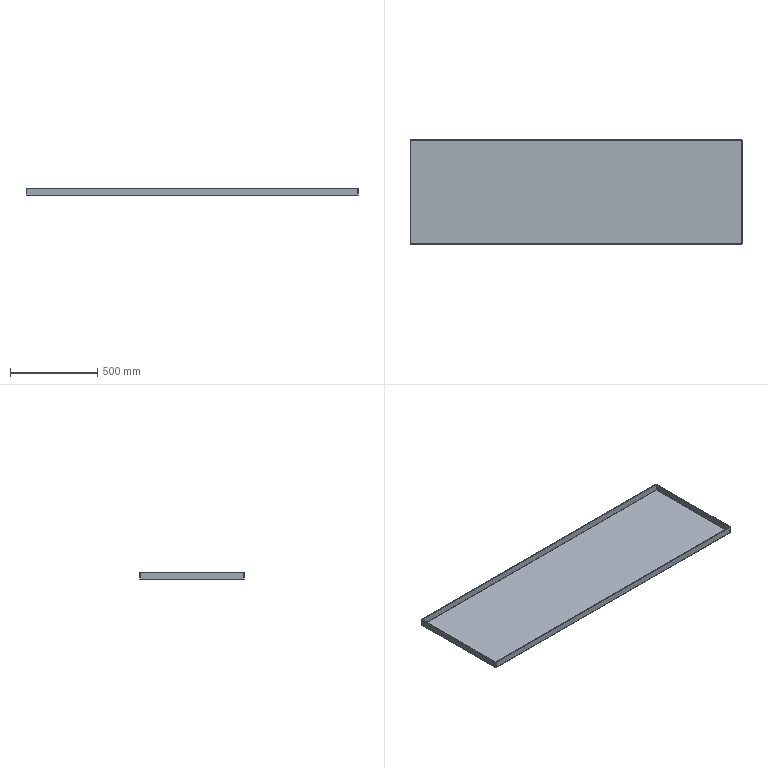Part | SolidWorks | features EdgeFlange 1, FlatPattern 1, SMBaseFlange 1, SheetMetal 1 | 1 solid | 38 faces | box 1900 x 600 x 40 mm | volume 2650874 mm3 | plane 22 | spline 8 | cylinder 8 | commonest cylinder face diameters 1.473 x4 5.473 x4
STEP:
#1=CARTESIAN_POINT('',(947.263,297.263,-2.));
#2=VERTEX_POINT('',#1);
#3=CARTESIAN_POINT('',(947.263,-297.263,-2.));
#4=VERTEX_POINT('',#3);
#5=CARTESIAN_POINT('',(947.263,297.293,-2.));
#6=DIRECTION('',(0.,-1.,0.));
#7=VECTOR('',#6,1000.);
#8=LINE('',#5,#7);
#9=EDGE_CURVE('',#2,#4,#8,.T.);
#10=ORIENTED_EDGE('',*,*,#9,.T.);
#11=CARTESIAN_POINT('',(-947.263,-297.263,-2.));
#12=VERTEX_POINT('',#11);
#13=CARTESIAN_POINT('',(947.293,-297.263,-2.));
#14=DIRECTION('',(-1.,0.,0.));
#15=VECTOR('',#14,1000.);
#16=LINE('',#13,#15);
#17=EDGE_CURVE('',#4,#12,#16,.T.);
#18=ORIENTED_EDGE('',*,*,#17,.T.);
#19=CARTESIAN_POINT('',(-947.263,297.263,-2.));
#20=VERTEX_POINT('',#19);
#21=CARTESIAN_POINT('',(-947.263,-297.293,-2.));
#22=DIRECTION('',(0.,1.,0.));
#23=VECTOR('',#22,1000.);
#24=LINE('',#21,#23);
#25=EDGE_CURVE('',#12,#20,#24,.T.);
#26=ORIENTED_EDGE('',*,*,#25,.T.);
#27=CARTESIAN_POINT('',(-947.293,297.263,-2.));
#28=DIRECTION('',(1.,0.,0.));
#29=VECTOR('',#28,1000.);
#30=LINE('',#27,#29);
#31=EDGE_CURVE('',#20,#2,#30,.T.);
#32=ORIENTED_EDGE('',*,*,#31,.T.);
#33=EDGE_LOOP('',(#10,#18,#26,#32));
#34=FACE_OUTER_BOUND('',#33,.T.);
#35=CARTESIAN_POINT('',(0.,0.,-2.));
#36=DIRECTION('',(0.,0.,-1.));
#37=DIRECTION('',(-1.,0.,0.));
#38=AXIS2_PLACEMENT_3D('',#35,#36,#37);
#39=PLANE('',#38);
#40=ADVANCED_FACE('',(#34),#39,.T.);
#41=CARTESIAN_POINT('',(947.263,-297.263,0.));
#42=VERTEX_POINT('',#41);
#43=CARTESIAN_POINT('',(-947.263,-297.263,0.));
#44=VERTEX_POINT('',#43);
#45=CARTESIAN_POINT('',(947.293,-297.263,0.));
#46=DIRECTION('',(-1.,0.,0.));
#47=VECTOR('',#46,1000.);
#48=LINE('',#45,#47);
#49=EDGE_CURVE('',#42,#44,#48,.T.);
#50=ORIENTED_EDGE('',*,*,#49,.F.);
#51=CARTESIAN_POINT('',(947.263,297.263,0.));
#52=VERTEX_POINT('',#51);
#53=CARTESIAN_POINT('',(947.263,297.293,0.));
#54=DIRECTION('',(0.,-1.,0.));
#55=VECTOR('',#54,1000.);
#56=LINE('',#53,#55);
#57=EDGE_CURVE('',#52,#42,#56,.T.);
#58=ORIENTED_EDGE('',*,*,#57,.F.);
#59=CARTESIAN_POINT('',(-947.263,297.263,0.));
#60=VERTEX_POINT('',#59);
#61=CARTESIAN_POINT('',(-947.293,297.263,0.));
#62=DIRECTION('',(1.,0.,0.));
#63=VECTOR('',#62,1000.);
#64=LINE('',#61,#63);
#65=EDGE_CURVE('',#60,#52,#64,.T.);
#66=ORIENTED_EDGE('',*,*,#65,.F.);
#67=CARTESIAN_POINT('',(-947.263,-297.293,0.));
#68=DIRECTION('',(0.,1.,0.));
#69=VECTOR('',#68,1000.);
#70=LINE('',#67,#69);
#71=EDGE_CURVE('',#44,#60,#70,.T.);
#72=ORIENTED_EDGE('',*,*,#71,.F.);
#73=EDGE_LOOP('',(#50,#58,#66,#72));
#74=FACE_OUTER_BOUND('',#73,.T.);
#75=CARTESIAN_POINT('',(0.,0.,0.));
#76=DIRECTION('',(0.,0.,-1.));
#77=DIRECTION('',(-1.,0.,0.));
#78=AXIS2_PLACEMENT_3D('',#75,#76,#77);
#79=PLANE('',#78);
#80=ADVANCED_FACE('',(#74),#79,.F.);
#81=CARTESIAN_POINT('',(947.293,300.,0.7366));
#82=VERTEX_POINT('',#81);
#83=CARTESIAN_POINT('',(947.293,298.,0.7366));
#84=VERTEX_POINT('',#83);
#85=CARTESIAN_POINT('',(947.293,298.,0.7366));
#86=DIRECTION('',(0.,-1.,0.));
#87=VECTOR('',#86,1000.);
#88=LINE('',#85,#87);
#89=EDGE_CURVE('',#82,#84,#88,.T.);
#90=ORIENTED_EDGE('',*,*,#89,.T.);
#91=CARTESIAN_POINT('',(947.263,297.263,0.));
#92=CARTESIAN_POINT('',(947.268,297.456,0.));
#93=CARTESIAN_POINT('',(947.273,297.648,0.07939));
#94=CARTESIAN_POINT('',(947.283,297.921,0.3521));
#95=CARTESIAN_POINT('',(947.288,298.,0.5438));
#96=CARTESIAN_POINT('',(947.293,298.,0.7366));
#97=B_SPLINE_CURVE_WITH_KNOTS('',3,(#91,#92,#93,#94,#95,#96),.UNSPECIFIED.,.F.,.F.,(4,2,4),(0.,0.5,1.),.UNSPECIFIED.);
#98=EDGE_CURVE('',#52,#84,#97,.T.);
#99=ORIENTED_EDGE('',*,*,#98,.F.);
#100=CARTESIAN_POINT('',(947.263,297.263,0.));
#101=DIRECTION('',(0.,0.,-1.));
#102=VECTOR('',#101,1000.);
#103=LINE('',#100,#102);
#104=EDGE_CURVE('',#52,#2,#103,.T.);
#105=ORIENTED_EDGE('',*,*,#104,.T.);
#106=CARTESIAN_POINT('',(947.263,297.263,-2.));
#107=CARTESIAN_POINT('',(947.266,297.622,-2.));
#108=CARTESIAN_POINT('',(947.268,297.98,-1.929));
#109=CARTESIAN_POINT('',(947.273,298.642,-1.655));
#110=CARTESIAN_POINT('',(947.276,298.945,-1.452));
#111=CARTESIAN_POINT('',(947.281,299.452,-0.9452));
#112=CARTESIAN_POINT('',(947.283,299.655,-0.6416));
#113=CARTESIAN_POINT('',(947.288,299.929,0.0203));
#114=CARTESIAN_POINT('',(947.29,300.,0.3784));
#115=CARTESIAN_POINT('',(947.293,300.,0.7366));
#116=B_SPLINE_CURVE_WITH_KNOTS('',3,(#106,#107,#108,#109,#110,#111,#112,#113,#114,#115),.UNSPECIFIED.,.F.,.F.,(4,2,2,2,4),(0.,0.25,0.5,0.75,1.),.UNSPECIFIED.);
#117=EDGE_CURVE('',#2,#82,#116,.T.);
#118=ORIENTED_EDGE('',*,*,#117,.T.);
#119=EDGE_LOOP('',(#90,#99,#105,#118));
#120=FACE_OUTER_BOUND('',#119,.T.);
#121=CARTESIAN_POINT('',(947.263,297.263,-2.02));
#122=CARTESIAN_POINT('',(947.266,297.624,-2.02));
#123=CARTESIAN_POINT('',(947.268,297.985,-1.948));
#124=CARTESIAN_POINT('',(947.273,298.652,-1.672));
#125=CARTESIAN_POINT('',(947.276,298.957,-1.468));
#126=CARTESIAN_POINT('',(947.281,299.468,-0.9575));
#127=CARTESIAN_POINT('',(947.283,299.672,-0.6517));
#128=CARTESIAN_POINT('',(947.288,299.948,0.01507));
#129=CARTESIAN_POINT('',(947.29,300.02,0.3757));
#130=CARTESIAN_POINT('',(947.293,300.02,0.7366));
#131=CARTESIAN_POINT('',(947.263,297.263,-2.));
#132=CARTESIAN_POINT('',(947.266,297.622,-2.));
#133=CARTESIAN_POINT('',(947.268,297.98,-1.929));
#134=CARTESIAN_POINT('',(947.273,298.642,-1.655));
#135=CARTESIAN_POINT('',(947.276,298.945,-1.452));
#136=CARTESIAN_POINT('',(947.281,299.452,-0.9452));
#137=CARTESIAN_POINT('',(947.283,299.655,-0.6416));
#138=CARTESIAN_POINT('',(947.288,299.929,0.0203));
#139=CARTESIAN_POINT('',(947.29,300.,0.3783));
#140=CARTESIAN_POINT('',(947.293,300.,0.7366));
#141=CARTESIAN_POINT('',(947.263,297.263,0.));
#142=CARTESIAN_POINT('',(947.266,297.36,0.));
#143=CARTESIAN_POINT('',(947.268,297.456,0.01917));
#144=CARTESIAN_POINT('',(947.273,297.634,0.09297));
#145=CARTESIAN_POINT('',(947.276,297.716,0.1476));
#146=CARTESIAN_POINT('',(947.281,297.852,0.2839));
#147=CARTESIAN_POINT('',(947.283,297.907,0.3656));
#148=CARTESIAN_POINT('',(947.288,297.981,0.5438));
#149=CARTESIAN_POINT('',(947.29,298.,0.6402));
#150=CARTESIAN_POINT('',(947.293,298.,0.7366));
#151=CARTESIAN_POINT('',(947.263,297.263,0.0202));
#152=CARTESIAN_POINT('',(947.266,297.357,0.0202));
#153=CARTESIAN_POINT('',(947.268,297.451,0.03885));
#154=CARTESIAN_POINT('',(947.273,297.624,0.1106));
#155=CARTESIAN_POINT('',(947.276,297.704,0.1637));
#156=CARTESIAN_POINT('',(947.281,297.836,0.2963));
#157=CARTESIAN_POINT('',(947.283,297.889,0.3758));
#158=CARTESIAN_POINT('',(947.288,297.961,0.5491));
#159=CARTESIAN_POINT('',(947.29,297.98,0.6428));
#160=CARTESIAN_POINT('',(947.293,297.98,0.7366));
#161=B_SPLINE_SURFACE_WITH_KNOTS('',1,3,((#121,#122,#123,#124,#125,#126,#127,#128,#129,#130),(#131,#132,#133,#134,#135,#136,#137,#138,#139,#140),(#141,#142,#143,#144,#145,#146,#147,#148,#149,#150),(#151,#152,#153,#154,#155,#156,#157,#158,#159,#160)),.UNSPECIFIED.,.F.,.F.,.F.,(2,1,1,2),(4,2,2,2,4),(-0.01,0.,1.,1.01),(0.,0.25,0.5,0.75,1.),.UNSPECIFIED.);
#162=ADVANCED_FACE('',(#120),#161,.F.);
#163=CARTESIAN_POINT('',(-947.293,298.,0.7366));
#164=VERTEX_POINT('',#163);
#165=CARTESIAN_POINT('',(-947.293,298.,0.7366));
#166=CARTESIAN_POINT('',(-947.288,298.,0.5438));
#167=CARTESIAN_POINT('',(-947.283,297.921,0.3521));
#168=CARTESIAN_POINT('',(-947.273,297.648,0.07939));
#169=CARTESIAN_POINT('',(-947.268,297.456,0.));
#170=CARTESIAN_POINT('',(-947.263,297.263,0.));
#171=B_SPLINE_CURVE_WITH_KNOTS('',3,(#165,#166,#167,#168,#169,#170),.UNSPECIFIED.,.F.,.F.,(4,2,4),(0.,0.5,1.),.UNSPECIFIED.);
#172=EDGE_CURVE('',#164,#60,#171,.T.);
#173=ORIENTED_EDGE('',*,*,#172,.F.);
#174=CARTESIAN_POINT('',(-947.293,300.,0.7366));
#175=VERTEX_POINT('',#174);
#176=CARTESIAN_POINT('',(-947.293,298.,0.7366));
#177=DIRECTION('',(0.,-1.,0.));
#178=VECTOR('',#177,1000.);
#179=LINE('',#176,#178);
#180=EDGE_CURVE('',#175,#164,#179,.T.);
#181=ORIENTED_EDGE('',*,*,#180,.F.);
#182=CARTESIAN_POINT('',(-947.293,300.,0.7366));
#183=CARTESIAN_POINT('',(-947.29,300.,0.3784));
#184=CARTESIAN_POINT('',(-947.288,299.929,0.0203));
#185=CARTESIAN_POINT('',(-947.283,299.655,-0.6416));
#186=CARTESIAN_POINT('',(-947.281,299.452,-0.9452));
#187=CARTESIAN_POINT('',(-947.276,298.945,-1.452));
#188=CARTESIAN_POINT('',(-947.273,298.642,-1.655));
#189=CARTESIAN_POINT('',(-947.268,297.98,-1.929));
#190=CARTESIAN_POINT('',(-947.266,297.622,-2.));
#191=CARTESIAN_POINT('',(-947.263,297.263,-2.));
#192=B_SPLINE_CURVE_WITH_KNOTS('',3,(#182,#183,#184,#185,#186,#187,#188,#189,#190,#191),.UNSPECIFIED.,.F.,.F.,(4,2,2,2,4),(0.,0.25,0.5,0.75,1.),.UNSPECIFIED.);
#193=EDGE_CURVE('',#175,#20,#192,.T.);
#194=ORIENTED_EDGE('',*,*,#193,.T.);
#195=CARTESIAN_POINT('',(-947.263,297.263,0.));
#196=DIRECTION('',(0.,0.,-1.));
#197=VECTOR('',#196,1000.);
#198=LINE('',#195,#197);
#199=EDGE_CURVE('',#60,#20,#198,.T.);
#200=ORIENTED_EDGE('',*,*,#199,.F.);
#201=EDGE_LOOP('',(#173,#181,#194,#200));
#202=FACE_OUTER_BOUND('',#201,.T.);
#203=CARTESIAN_POINT('',(-947.293,300.02,0.7366));
#204=CARTESIAN_POINT('',(-947.29,300.02,0.3757));
#205=CARTESIAN_POINT('',(-947.288,299.948,0.01507));
#206=CARTESIAN_POINT('',(-947.283,299.672,-0.6517));
#207=CARTESIAN_POINT('',(-947.281,299.468,-0.9575));
#208=CARTESIAN_POINT('',(-947.276,298.957,-1.468));
#209=CARTESIAN_POINT('',(-947.273,298.652,-1.672));
#210=CARTESIAN_POINT('',(-947.268,297.985,-1.948));
#211=CARTESIAN_POINT('',(-947.266,297.624,-2.02));
#212=CARTESIAN_POINT('',(-947.263,297.263,-2.02));
#213=CARTESIAN_POINT('',(-947.293,300.,0.7366));
#214=CARTESIAN_POINT('',(-947.29,300.,0.3783));
#215=CARTESIAN_POINT('',(-947.288,299.929,0.0203));
#216=CARTESIAN_POINT('',(-947.283,299.655,-0.6416));
#217=CARTESIAN_POINT('',(-947.281,299.452,-0.9452));
#218=CARTESIAN_POINT('',(-947.276,298.945,-1.452));
#219=CARTESIAN_POINT('',(-947.273,298.642,-1.655));
#220=CARTESIAN_POINT('',(-947.268,297.98,-1.929));
#221=CARTESIAN_POINT('',(-947.266,297.622,-2.));
#222=CARTESIAN_POINT('',(-947.263,297.263,-2.));
#223=CARTESIAN_POINT('',(-947.293,298.,0.7366));
#224=CARTESIAN_POINT('',(-947.29,298.,0.6402));
#225=CARTESIAN_POINT('',(-947.288,297.981,0.5438));
#226=CARTESIAN_POINT('',(-947.283,297.907,0.3656));
#227=CARTESIAN_POINT('',(-947.281,297.852,0.2839));
#228=CARTESIAN_POINT('',(-947.276,297.716,0.1476));
#229=CARTESIAN_POINT('',(-947.273,297.634,0.09297));
#230=CARTESIAN_POINT('',(-947.268,297.456,0.01917));
#231=CARTESIAN_POINT('',(-947.266,297.36,0.));
#232=CARTESIAN_POINT('',(-947.263,297.263,0.));
#233=CARTESIAN_POINT('',(-947.293,297.98,0.7366));
#234=CARTESIAN_POINT('',(-947.29,297.98,0.6428));
#235=CARTESIAN_POINT('',(-947.288,297.961,0.5491));
#236=CARTESIAN_POINT('',(-947.283,297.889,0.3758));
#237=CARTESIAN_POINT('',(-947.281,297.836,0.2963));
#238=CARTESIAN_POINT('',(-947.276,297.704,0.1637));
#239=CARTESIAN_POINT('',(-947.273,297.624,0.1106));
#240=CARTESIAN_POINT('',(-947.268,297.451,0.03885));
#241=CARTESIAN_POINT('',(-947.266,297.357,0.0202));
#242=CARTESIAN_POINT('',(-947.263,297.263,0.0202));
#243=B_SPLINE_SURFACE_WITH_KNOTS('',1,3,((#203,#204,#205,#206,#207,#208,#209,#210,#211,#212),(#213,#214,#215,#216,#217,#218,#219,#220,#221,#222),(#223,#224,#225,#226,#227,#228,#229,#230,#231,#232),(#233,#234,#235,#236,#237,#238,#239,#240,#241,#242)),.UNSPECIFIED.,.F.,.F.,.F.,(2,1,1,2),(4,2,2,2,4),(-0.01,0.,1.,1.01),(0.,0.25,0.5,0.75,1.),.UNSPECIFIED.);
#244=ADVANCED_FACE('',(#202),#243,.F.);
#245=ORIENTED_EDGE('',*,*,#31,.F.);
#246=ORIENTED_EDGE('',*,*,#193,.F.);
#247=CARTESIAN_POINT('',(0.,300.,0.7366));
#248=DIRECTION('',(-1.,0.,0.));
#249=VECTOR('',#248,1000.);
#250=LINE('',#247,#249);
#251=EDGE_CURVE('',#82,#175,#250,.T.);
#252=ORIENTED_EDGE('',*,*,#251,.F.);
#253=ORIENTED_EDGE('',*,*,#117,.F.);
#254=EDGE_LOOP('',(#245,#246,#252,#253));
#255=FACE_OUTER_BOUND('',#254,.T.);
#256=CARTESIAN_POINT('',(-947.293,297.263,0.7366));
#257=DIRECTION('',(-1.,0.,0.));
#258=DIRECTION('',(0.,1.,0.));
#259=AXIS2_PLACEMENT_3D('',#256,#257,#258);
#260=CYLINDRICAL_SURFACE('',#259,2.737);
#261=ADVANCED_FACE('',(#255),#260,.T.);
#262=ORIENTED_EDGE('',*,*,#65,.T.);
#263=ORIENTED_EDGE('',*,*,#98,.T.);
#264=CARTESIAN_POINT('',(950.,298.,0.7366));
#265=DIRECTION('',(-1.,0.,0.));
#266=VECTOR('',#265,1000.);
#267=LINE('',#264,#266);
#268=EDGE_CURVE('',#84,#164,#267,.T.);
#269=ORIENTED_EDGE('',*,*,#268,.T.);
#270=ORIENTED_EDGE('',*,*,#172,.T.);
#271=EDGE_LOOP('',(#262,#263,#269,#270));
#272=FACE_OUTER_BOUND('',#271,.T.);
#273=CARTESIAN_POINT('',(-947.293,297.263,0.7366));
#274=DIRECTION('',(-1.,0.,0.));
#275=DIRECTION('',(0.,1.,0.));
#276=AXIS2_PLACEMENT_3D('',#273,#274,#275);
#277=CYLINDRICAL_SURFACE('',#276,0.7366);
#278=ADVANCED_FACE('',(#272),#277,.F.);
#279=CARTESIAN_POINT('',(947.293,298.,38.));
#280=VERTEX_POINT('',#279);
#281=CARTESIAN_POINT('',(947.293,300.,38.));
#282=VERTEX_POINT('',#281);
#283=CARTESIAN_POINT('',(947.293,300.,38.));
#284=DIRECTION('',(0.,1.,0.));
#285=VECTOR('',#284,1000.);
#286=LINE('',#283,#285);
#287=EDGE_CURVE('',#280,#282,#286,.T.);
#288=ORIENTED_EDGE('',*,*,#287,.F.);
#289=CARTESIAN_POINT('',(947.293,298.,0.));
#290=DIRECTION('',(0.,0.,1.));
#291=VECTOR('',#290,1000.);
#292=LINE('',#289,#291);
#293=EDGE_CURVE('',#84,#280,#292,.T.);
#294=ORIENTED_EDGE('',*,*,#293,.F.);
#295=ORIENTED_EDGE('',*,*,#89,.F.);
#296=CARTESIAN_POINT('',(947.293,300.,0.));
#297=DIRECTION('',(0.,0.,-1.));
#298=VECTOR('',#297,1000.);
#299=LINE('',#296,#298);
#300=EDGE_CURVE('',#282,#82,#299,.T.);
#301=ORIENTED_EDGE('',*,*,#300,.F.);
#302=EDGE_LOOP('',(#288,#294,#295,#301));
#303=FACE_OUTER_BOUND('',#302,.T.);
#304=CARTESIAN_POINT('',(947.293,298.,0.));
#305=DIRECTION('',(1.,0.,0.));
#306=DIRECTION('',(0.,0.,-1.));
#307=AXIS2_PLACEMENT_3D('',#304,#305,#306);
#308=PLANE('',#307);
#309=ADVANCED_FACE('',(#303),#308,.T.);
#310=CARTESIAN_POINT('',(-947.293,300.,38.));
#311=VERTEX_POINT('',#310);
#312=CARTESIAN_POINT('',(-947.293,300.,0.));
#313=DIRECTION('',(0.,0.,-1.));
#314=VECTOR('',#313,1000.);
#315=LINE('',#312,#314);
#316=EDGE_CURVE('',#311,#175,#315,.T.);
#317=ORIENTED_EDGE('',*,*,#316,.F.);
#318=CARTESIAN_POINT('',(-950.,300.,38.));
#319=DIRECTION('',(-1.,0.,0.));
#320=VECTOR('',#319,1000.);
#321=LINE('',#318,#320);
#322=EDGE_CURVE('',#282,#311,#321,.T.);
#323=ORIENTED_EDGE('',*,*,#322,.F.);
#324=ORIENTED_EDGE('',*,*,#300,.T.);
#325=ORIENTED_EDGE('',*,*,#251,.T.);
#326=EDGE_LOOP('',(#317,#323,#324,#325));
#327=FACE_OUTER_BOUND('',#326,.T.);
#328=CARTESIAN_POINT('',(0.,300.,0.));
#329=DIRECTION('',(0.,1.,0.));
#330=DIRECTION('',(0.,0.,1.));
#331=AXIS2_PLACEMENT_3D('',#328,#329,#330);
#332=PLANE('',#331);
#333=ADVANCED_FACE('',(#327),#332,.T.);
#334=CARTESIAN_POINT('',(-947.293,298.,38.));
#335=VERTEX_POINT('',#334);
#336=CARTESIAN_POINT('',(0.,298.,38.));
#337=DIRECTION('',(-1.,0.,0.));
#338=VECTOR('',#337,1000.);
#339=LINE('',#336,#338);
#340=EDGE_CURVE('',#280,#335,#339,.T.);
#341=ORIENTED_EDGE('',*,*,#340,.T.);
#342=CARTESIAN_POINT('',(-947.293,298.,0.));
#343=DIRECTION('',(0.,0.,1.));
#344=VECTOR('',#343,1000.);
#345=LINE('',#342,#344);
#346=EDGE_CURVE('',#164,#335,#345,.T.);
#347=ORIENTED_EDGE('',*,*,#346,.F.);
#348=ORIENTED_EDGE('',*,*,#268,.F.);
#349=ORIENTED_EDGE('',*,*,#293,.T.);
#350=EDGE_LOOP('',(#341,#347,#348,#349));
#351=FACE_OUTER_BOUND('',#350,.T.);
#352=CARTESIAN_POINT('',(0.,298.,0.));
#353=DIRECTION('',(0.,1.,0.));
#354=DIRECTION('',(0.,0.,1.));
#355=AXIS2_PLACEMENT_3D('',#352,#353,#354);
#356=PLANE('',#355);
#357=ADVANCED_FACE('',(#351),#356,.F.);
#358=CARTESIAN_POINT('',(-947.293,298.,38.));
#359=DIRECTION('',(0.,1.,0.));
#360=VECTOR('',#359,1000.);
#361=LINE('',#358,#360);
#362=EDGE_CURVE('',#335,#311,#361,.T.);
#363=ORIENTED_EDGE('',*,*,#362,.F.);
#364=ORIENTED_EDGE('',*,*,#340,.F.);
#365=ORIENTED_EDGE('',*,*,#287,.T.);
#366=ORIENTED_EDGE('',*,*,#322,.T.);
#367=EDGE_LOOP('',(#363,#364,#365,#366));
#368=FACE_OUTER_BOUND('',#367,.T.);
#369=CARTESIAN_POINT('',(-950.,300.,38.));
#370=DIRECTION('',(0.,0.,1.));
#371=DIRECTION('',(0.,-1.,0.));
#372=AXIS2_PLACEMENT_3D('',#369,#370,#371);
#373=PLANE('',#372);
#374=ADVANCED_FACE('',(#368),#373,.T.);
#375=ORIENTED_EDGE('',*,*,#346,.T.);
#376=ORIENTED_EDGE('',*,*,#362,.T.);
#377=ORIENTED_EDGE('',*,*,#316,.T.);
#378=ORIENTED_EDGE('',*,*,#180,.T.);
#379=EDGE_LOOP('',(#375,#376,#377,#378));
#380=FACE_OUTER_BOUND('',#379,.T.);
#381=CARTESIAN_POINT('',(-947.293,298.,0.));
#382=DIRECTION('',(1.,0.,0.));
#383=DIRECTION('',(0.,0.,-1.));
#384=AXIS2_PLACEMENT_3D('',#381,#382,#383);
#385=PLANE('',#384);
#386=ADVANCED_FACE('',(#380),#385,.F.);
#387=CARTESIAN_POINT('',(-950.,297.293,0.7366));
#388=VERTEX_POINT('',#387);
#389=CARTESIAN_POINT('',(-948.,297.293,0.7366));
#390=VERTEX_POINT('',#389);
#391=CARTESIAN_POINT('',(-948.,297.293,0.7366));
#392=DIRECTION('',(1.,0.,0.));
#393=VECTOR('',#392,1000.);
#394=LINE('',#391,#393);
#395=EDGE_CURVE('',#388,#390,#394,.T.);
#396=ORIENTED_EDGE('',*,*,#395,.T.);
#397=CARTESIAN_POINT('',(-947.263,297.263,0.));
#398=CARTESIAN_POINT('',(-947.456,297.268,0.));
#399=CARTESIAN_POINT('',(-947.648,297.273,0.07939));
#400=CARTESIAN_POINT('',(-947.921,297.283,0.3521));
#401=CARTESIAN_POINT('',(-948.,297.288,0.5438));
#402=CARTESIAN_POINT('',(-948.,297.293,0.7366));
#403=B_SPLINE_CURVE_WITH_KNOTS('',3,(#397,#398,#399,#400,#401,#402),.UNSPECIFIED.,.F.,.F.,(4,2,4),(0.,0.5,1.),.UNSPECIFIED.);
#404=EDGE_CURVE('',#60,#390,#403,.T.);
#405=ORIENTED_EDGE('',*,*,#404,.F.);
#406=ORIENTED_EDGE('',*,*,#199,.T.);
#407=CARTESIAN_POINT('',(-947.263,297.263,-2.));
#408=CARTESIAN_POINT('',(-947.622,297.266,-2.));
#409=CARTESIAN_POINT('',(-947.98,297.268,-1.929));
#410=CARTESIAN_POINT('',(-948.642,297.273,-1.655));
#411=CARTESIAN_POINT('',(-948.945,297.276,-1.452));
#412=CARTESIAN_POINT('',(-949.452,297.281,-0.9452));
#413=CARTESIAN_POINT('',(-949.655,297.283,-0.6416));
#414=CARTESIAN_POINT('',(-949.929,297.288,0.0203));
#415=CARTESIAN_POINT('',(-950.,297.29,0.3784));
#416=CARTESIAN_POINT('',(-950.,297.293,0.7366));
#417=B_SPLINE_CURVE_WITH_KNOTS('',3,(#407,#408,#409,#410,#411,#412,#413,#414,#415,#416),.UNSPECIFIED.,.F.,.F.,(4,2,2,2,4),(0.,0.25,0.5,0.75,1.),.UNSPECIFIED.);
#418=EDGE_CURVE('',#20,#388,#417,.T.);
#419=ORIENTED_EDGE('',*,*,#418,.T.);
#420=EDGE_LOOP('',(#396,#405,#406,#419));
#421=FACE_OUTER_BOUND('',#420,.T.);
#422=CARTESIAN_POINT('',(-947.263,297.263,-2.02));
#423=CARTESIAN_POINT('',(-947.624,297.266,-2.02));
#424=CARTESIAN_POINT('',(-947.985,297.268,-1.948));
#425=CARTESIAN_POINT('',(-948.652,297.273,-1.672));
#426=CARTESIAN_POINT('',(-948.957,297.276,-1.468));
#427=CARTESIAN_POINT('',(-949.468,297.281,-0.9575));
#428=CARTESIAN_POINT('',(-949.672,297.283,-0.6517));
#429=CARTESIAN_POINT('',(-949.948,297.288,0.01507));
#430=CARTESIAN_POINT('',(-950.02,297.29,0.3757));
#431=CARTESIAN_POINT('',(-950.02,297.293,0.7366));
#432=CARTESIAN_POINT('',(-947.263,297.263,-2.));
#433=CARTESIAN_POINT('',(-947.622,297.266,-2.));
#434=CARTESIAN_POINT('',(-947.98,297.268,-1.929));
#435=CARTESIAN_POINT('',(-948.642,297.273,-1.655));
#436=CARTESIAN_POINT('',(-948.945,297.276,-1.452));
#437=CARTESIAN_POINT('',(-949.452,297.281,-0.9452));
#438=CARTESIAN_POINT('',(-949.655,297.283,-0.6416));
#439=CARTESIAN_POINT('',(-949.929,297.288,0.0203));
#440=CARTESIAN_POINT('',(-950.,297.29,0.3783));
#441=CARTESIAN_POINT('',(-950.,297.293,0.7366));
#442=CARTESIAN_POINT('',(-947.263,297.263,0.));
#443=CARTESIAN_POINT('',(-947.36,297.266,0.));
#444=CARTESIAN_POINT('',(-947.456,297.268,0.01917));
#445=CARTESIAN_POINT('',(-947.634,297.273,0.09297));
#446=CARTESIAN_POINT('',(-947.716,297.276,0.1476));
#447=CARTESIAN_POINT('',(-947.852,297.281,0.2839));
#448=CARTESIAN_POINT('',(-947.907,297.283,0.3656));
#449=CARTESIAN_POINT('',(-947.981,297.288,0.5438));
#450=CARTESIAN_POINT('',(-948.,297.29,0.6402));
#451=CARTESIAN_POINT('',(-948.,297.293,0.7366));
#452=CARTESIAN_POINT('',(-947.263,297.263,0.0202));
#453=CARTESIAN_POINT('',(-947.357,297.266,0.0202));
#454=CARTESIAN_POINT('',(-947.451,297.268,0.03885));
#455=CARTESIAN_POINT('',(-947.624,297.273,0.1106));
#456=CARTESIAN_POINT('',(-947.704,297.276,0.1637));
#457=CARTESIAN_POINT('',(-947.836,297.281,0.2963));
#458=CARTESIAN_POINT('',(-947.889,297.283,0.3758));
#459=CARTESIAN_POINT('',(-947.961,297.288,0.5491));
#460=CARTESIAN_POINT('',(-947.98,297.29,0.6428));
#461=CARTESIAN_POINT('',(-947.98,297.293,0.7366));
#462=B_SPLINE_SURFACE_WITH_KNOTS('',1,3,((#422,#423,#424,#425,#426,#427,#428,#429,#430,#431),(#432,#433,#434,#435,#436,#437,#438,#439,#440,#441),(#442,#443,#444,#445,#446,#447,#448,#449,#450,#451),(#452,#453,#454,#455,#456,#457,#458,#459,#460,#461)),.UNSPECIFIED.,.F.,.F.,.F.,(2,1,1,2),(4,2,2,2,4),(-0.01,0.,1.,1.01),(0.,0.25,0.5,0.75,1.),.UNSPECIFIED.);
#463=ADVANCED_FACE('',(#421),#462,.F.);
#464=CARTESIAN_POINT('',(-948.,-297.293,0.7366));
#465=VERTEX_POINT('',#464);
#466=CARTESIAN_POINT('',(-948.,-297.293,0.7366));
#467=CARTESIAN_POINT('',(-948.,-297.288,0.5438));
#468=CARTESIAN_POINT('',(-947.921,-297.283,0.3521));
#469=CARTESIAN_POINT('',(-947.648,-297.273,0.07939));
#470=CARTESIAN_POINT('',(-947.456,-297.268,0.));
#471=CARTESIAN_POINT('',(-947.263,-297.263,0.));
#472=B_SPLINE_CURVE_WITH_KNOTS('',3,(#466,#467,#468,#469,#470,#471),.UNSPECIFIED.,.F.,.F.,(4,2,4),(0.,0.5,1.),.UNSPECIFIED.);
#473=EDGE_CURVE('',#465,#44,#472,.T.);
#474=ORIENTED_EDGE('',*,*,#473,.F.);
#475=CARTESIAN_POINT('',(-950.,-297.293,0.7366));
#476=VERTEX_POINT('',#475);
#477=CARTESIAN_POINT('',(-948.,-297.293,0.7366));
#478=DIRECTION('',(1.,0.,0.));
#479=VECTOR('',#478,1000.);
#480=LINE('',#477,#479);
#481=EDGE_CURVE('',#476,#465,#480,.T.);
#482=ORIENTED_EDGE('',*,*,#481,.F.);
#483=CARTESIAN_POINT('',(-950.,-297.293,0.7366));
#484=CARTESIAN_POINT('',(-950.,-297.29,0.3784));
#485=CARTESIAN_POINT('',(-949.929,-297.288,0.0203));
#486=CARTESIAN_POINT('',(-949.655,-297.283,-0.6416));
#487=CARTESIAN_POINT('',(-949.452,-297.281,-0.9452));
#488=CARTESIAN_POINT('',(-948.945,-297.276,-1.452));
#489=CARTESIAN_POINT('',(-948.642,-297.273,-1.655));
#490=CARTESIAN_POINT('',(-947.98,-297.268,-1.929));
#491=CARTESIAN_POINT('',(-947.622,-297.266,-2.));
#492=CARTESIAN_POINT('',(-947.263,-297.263,-2.));
#493=B_SPLINE_CURVE_WITH_KNOTS('',3,(#483,#484,#485,#486,#487,#488,#489,#490,#491,#492),.UNSPECIFIED.,.F.,.F.,(4,2,2,2,4),(0.,0.25,0.5,0.75,1.),.UNSPECIFIED.);
#494=EDGE_CURVE('',#476,#12,#493,.T.);
#495=ORIENTED_EDGE('',*,*,#494,.T.);
#496=CARTESIAN_POINT('',(-947.263,-297.263,0.));
#497=DIRECTION('',(0.,0.,-1.));
#498=VECTOR('',#497,1000.);
#499=LINE('',#496,#498);
#500=EDGE_CURVE('',#44,#12,#499,.T.);
#501=ORIENTED_EDGE('',*,*,#500,.F.);
#502=EDGE_LOOP('',(#474,#482,#495,#501));
#503=FACE_OUTER_BOUND('',#502,.T.);
#504=CARTESIAN_POINT('',(-950.02,-297.293,0.7366));
#505=CARTESIAN_POINT('',(-950.02,-297.29,0.3757));
#506=CARTESIAN_POINT('',(-949.948,-297.288,0.01507));
#507=CARTESIAN_POINT('',(-949.672,-297.283,-0.6517));
#508=CARTESIAN_POINT('',(-949.468,-297.281,-0.9575));
#509=CARTESIAN_POINT('',(-948.957,-297.276,-1.468));
#510=CARTESIAN_POINT('',(-948.652,-297.273,-1.672));
#511=CARTESIAN_POINT('',(-947.985,-297.268,-1.948));
#512=CARTESIAN_POINT('',(-947.624,-297.266,-2.02));
#513=CARTESIAN_POINT('',(-947.263,-297.263,-2.02));
#514=CARTESIAN_POINT('',(-950.,-297.293,0.7366));
#515=CARTESIAN_POINT('',(-950.,-297.29,0.3783));
#516=CARTESIAN_POINT('',(-949.929,-297.288,0.0203));
#517=CARTESIAN_POINT('',(-949.655,-297.283,-0.6416));
#518=CARTESIAN_POINT('',(-949.452,-297.281,-0.9452));
#519=CARTESIAN_POINT('',(-948.945,-297.276,-1.452));
#520=CARTESIAN_POINT('',(-948.642,-297.273,-1.655));
#521=CARTESIAN_POINT('',(-947.98,-297.268,-1.929));
#522=CARTESIAN_POINT('',(-947.622,-297.266,-2.));
#523=CARTESIAN_POINT('',(-947.263,-297.263,-2.));
#524=CARTESIAN_POINT('',(-948.,-297.293,0.7366));
#525=CARTESIAN_POINT('',(-948.,-297.29,0.6402));
#526=CARTESIAN_POINT('',(-947.981,-297.288,0.5438));
#527=CARTESIAN_POINT('',(-947.907,-297.283,0.3656));
#528=CARTESIAN_POINT('',(-947.852,-297.281,0.2839));
#529=CARTESIAN_POINT('',(-947.716,-297.276,0.1476));
#530=CARTESIAN_POINT('',(-947.634,-297.273,0.09297));
#531=CARTESIAN_POINT('',(-947.456,-297.268,0.01917));
#532=CARTESIAN_POINT('',(-947.36,-297.266,0.));
#533=CARTESIAN_POINT('',(-947.263,-297.263,0.));
#534=CARTESIAN_POINT('',(-947.98,-297.293,0.7366));
#535=CARTESIAN_POINT('',(-947.98,-297.29,0.6428));
#536=CARTESIAN_POINT('',(-947.961,-297.288,0.5491));
#537=CARTESIAN_POINT('',(-947.889,-297.283,0.3758));
#538=CARTESIAN_POINT('',(-947.836,-297.281,0.2963));
#539=CARTESIAN_POINT('',(-947.704,-297.276,0.1637));
#540=CARTESIAN_POINT('',(-947.624,-297.273,0.1106));
#541=CARTESIAN_POINT('',(-947.451,-297.268,0.03885));
#542=CARTESIAN_POINT('',(-947.357,-297.266,0.0202));
#543=CARTESIAN_POINT('',(-947.263,-297.263,0.0202));
#544=B_SPLINE_SURFACE_WITH_KNOTS('',1,3,((#504,#505,#506,#507,#508,#509,#510,#511,#512,#513),(#514,#515,#516,#517,#518,#519,#520,#521,#522,#523),(#524,#525,#526,#527,#528,#529,#530,#531,#532,#533),(#534,#535,#536,#537,#538,#539,#540,#541,#542,#543)),.UNSPECIFIED.,.F.,.F.,.F.,(2,1,1,2),(4,2,2,2,4),(-0.01,0.,1.,1.01),(0.,0.25,0.5,0.75,1.),.UNSPECIFIED.);
#545=ADVANCED_FACE('',(#503),#544,.F.);
#546=ORIENTED_EDGE('',*,*,#25,.F.);
#547=ORIENTED_EDGE('',*,*,#494,.F.);
#548=CARTESIAN_POINT('',(-950.,300.,0.7366));
#549=DIRECTION('',(0.,1.,0.));
#550=VECTOR('',#549,1000.);
#551=LINE('',#548,#550);
#552=EDGE_CURVE('',#476,#388,#551,.T.);
#553=ORIENTED_EDGE('',*,*,#552,.T.);
#554=ORIENTED_EDGE('',*,*,#418,.F.);
#555=EDGE_LOOP('',(#546,#547,#553,#554));
#556=FACE_OUTER_BOUND('',#555,.T.);
#557=CARTESIAN_POINT('',(-947.263,-297.293,0.7366));
#558=DIRECTION('',(0.,-1.,0.));
#559=DIRECTION('',(-1.,0.,0.));
#560=AXIS2_PLACEMENT_3D('',#557,#558,#559);
#561=CYLINDRICAL_SURFACE('',#560,2.737);
#562=ADVANCED_FACE('',(#556),#561,.T.);
#563=ORIENTED_EDGE('',*,*,#71,.T.);
#564=ORIENTED_EDGE('',*,*,#404,.T.);
#565=CARTESIAN_POINT('',(-948.,300.,0.7366));
#566=DIRECTION('',(0.,-1.,0.));
#567=VECTOR('',#566,1000.);
#568=LINE('',#565,#567);
#569=EDGE_CURVE('',#390,#465,#568,.T.);
#570=ORIENTED_EDGE('',*,*,#569,.T.);
#571=ORIENTED_EDGE('',*,*,#473,.T.);
#572=EDGE_LOOP('',(#563,#564,#570,#571));
#573=FACE_OUTER_BOUND('',#572,.T.);
#574=CARTESIAN_POINT('',(-947.263,-297.293,0.7366));
#575=DIRECTION('',(0.,-1.,0.));
#576=DIRECTION('',(-1.,0.,0.));
#577=AXIS2_PLACEMENT_3D('',#574,#575,#576);
#578=CYLINDRICAL_SURFACE('',#577,0.7366);
#579=ADVANCED_FACE('',(#573),#578,.F.);
#580=CARTESIAN_POINT('',(-948.,297.293,38.));
#581=VERTEX_POINT('',#580);
#582=CARTESIAN_POINT('',(-950.,297.293,38.));
#583=VERTEX_POINT('',#582);
#584=CARTESIAN_POINT('',(-950.,297.293,38.));
#585=DIRECTION('',(-1.,0.,0.));
#586=VECTOR('',#585,1000.);
#587=LINE('',#584,#586);
#588=EDGE_CURVE('',#581,#583,#587,.T.);
#589=ORIENTED_EDGE('',*,*,#588,.F.);
#590=CARTESIAN_POINT('',(-948.,297.293,0.));
#591=DIRECTION('',(0.,0.,1.));
#592=VECTOR('',#591,1000.);
#593=LINE('',#590,#592);
#594=EDGE_CURVE('',#390,#581,#593,.T.);
#595=ORIENTED_EDGE('',*,*,#594,.F.);
#596=ORIENTED_EDGE('',*,*,#395,.F.);
#597=CARTESIAN_POINT('',(-950.,297.293,0.));
#598=DIRECTION('',(0.,0.,1.));
#599=VECTOR('',#598,1000.);
#600=LINE('',#597,#599);
#601=EDGE_CURVE('',#388,#583,#600,.T.);
#602=ORIENTED_EDGE('',*,*,#601,.T.);
#603=EDGE_LOOP('',(#589,#595,#596,#602));
#604=FACE_OUTER_BOUND('',#603,.T.);
#605=CARTESIAN_POINT('',(-948.,297.293,0.));
#606=DIRECTION('',(0.,1.,0.));
#607=DIRECTION('',(0.,0.,1.));
#608=AXIS2_PLACEMENT_3D('',#605,#606,#607);
#609=PLANE('',#608);
#610=ADVANCED_FACE('',(#604),#609,.T.);
#611=ORIENTED_EDGE('',*,*,#552,.F.);
#612=CARTESIAN_POINT('',(-950.,-297.293,38.));
#613=VERTEX_POINT('',#612);
#614=CARTESIAN_POINT('',(-950.,-297.293,0.));
#615=DIRECTION('',(0.,0.,1.));
#616=VECTOR('',#615,1000.);
#617=LINE('',#614,#616);
#618=EDGE_CURVE('',#476,#613,#617,.T.);
#619=ORIENTED_EDGE('',*,*,#618,.T.);
#620=CARTESIAN_POINT('',(-950.,300.,38.));
#621=DIRECTION('',(0.,-1.,0.));
#622=VECTOR('',#621,1000.);
#623=LINE('',#620,#622);
#624=EDGE_CURVE('',#583,#613,#623,.T.);
#625=ORIENTED_EDGE('',*,*,#624,.F.);
#626=ORIENTED_EDGE('',*,*,#601,.F.);
#627=EDGE_LOOP('',(#611,#619,#625,#626));
#628=FACE_OUTER_BOUND('',#627,.T.);
#629=CARTESIAN_POINT('',(-950.,0.,0.));
#630=DIRECTION('',(1.,0.,0.));
#631=DIRECTION('',(0.,0.,-1.));
#632=AXIS2_PLACEMENT_3D('',#629,#630,#631);
#633=PLANE('',#632);
#634=ADVANCED_FACE('',(#628),#633,.F.);
#635=CARTESIAN_POINT('',(-948.,-297.293,38.));
#636=VERTEX_POINT('',#635);
#637=CARTESIAN_POINT('',(-948.,-297.293,0.));
#638=DIRECTION('',(0.,0.,1.));
#639=VECTOR('',#638,1000.);
#640=LINE('',#637,#639);
#641=EDGE_CURVE('',#465,#636,#640,.T.);
#642=ORIENTED_EDGE('',*,*,#641,.F.);
#643=ORIENTED_EDGE('',*,*,#569,.F.);
#644=ORIENTED_EDGE('',*,*,#594,.T.);
#645=CARTESIAN_POINT('',(-948.,0.,38.));
#646=DIRECTION('',(0.,-1.,0.));
#647=VECTOR('',#646,1000.);
#648=LINE('',#645,#647);
#649=EDGE_CURVE('',#581,#636,#648,.T.);
#650=ORIENTED_EDGE('',*,*,#649,.T.);
#651=EDGE_LOOP('',(#642,#643,#644,#650));
#652=FACE_OUTER_BOUND('',#651,.T.);
#653=CARTESIAN_POINT('',(-948.,0.,0.));
#654=DIRECTION('',(1.,0.,0.));
#655=DIRECTION('',(0.,0.,-1.));
#656=AXIS2_PLACEMENT_3D('',#653,#654,#655);
#657=PLANE('',#656);
#658=ADVANCED_FACE('',(#652),#657,.T.);
#659=CARTESIAN_POINT('',(-948.,-297.293,38.));
#660=DIRECTION('',(-1.,0.,0.));
#661=VECTOR('',#660,1000.);
#662=LINE('',#659,#661);
#663=EDGE_CURVE('',#636,#613,#662,.T.);
#664=ORIENTED_EDGE('',*,*,#663,.F.);
#665=ORIENTED_EDGE('',*,*,#649,.F.);
#666=ORIENTED_EDGE('',*,*,#588,.T.);
#667=ORIENTED_EDGE('',*,*,#624,.T.);
#668=EDGE_LOOP('',(#664,#665,#666,#667));
#669=FACE_OUTER_BOUND('',#668,.T.);
#670=CARTESIAN_POINT('',(-950.,300.,38.));
#671=DIRECTION('',(0.,0.,1.));
#672=DIRECTION('',(1.,0.,0.));
#673=AXIS2_PLACEMENT_3D('',#670,#671,#672);
#674=PLANE('',#673);
#675=ADVANCED_FACE('',(#669),#674,.T.);
#676=ORIENTED_EDGE('',*,*,#641,.T.);
#677=ORIENTED_EDGE('',*,*,#663,.T.);
#678=ORIENTED_EDGE('',*,*,#618,.F.);
#679=ORIENTED_EDGE('',*,*,#481,.T.);
#680=EDGE_LOOP('',(#676,#677,#678,#679));
#681=FACE_OUTER_BOUND('',#680,.T.);
#682=CARTESIAN_POINT('',(-948.,-297.293,0.));
#683=DIRECTION('',(0.,1.,0.));
#684=DIRECTION('',(0.,0.,1.));
#685=AXIS2_PLACEMENT_3D('',#682,#683,#684);
#686=PLANE('',#685);
#687=ADVANCED_FACE('',(#681),#686,.F.);
#688=CARTESIAN_POINT('',(950.,-297.293,0.7366));
#689=VERTEX_POINT('',#688);
#690=CARTESIAN_POINT('',(948.,-297.293,0.7366));
#691=VERTEX_POINT('',#690);
#692=CARTESIAN_POINT('',(948.,-297.293,0.7366));
#693=DIRECTION('',(-1.,0.,0.));
#694=VECTOR('',#693,1000.);
#695=LINE('',#692,#694);
#696=EDGE_CURVE('',#689,#691,#695,.T.);
#697=ORIENTED_EDGE('',*,*,#696,.T.);
#698=CARTESIAN_POINT('',(947.263,-297.263,0.));
#699=CARTESIAN_POINT('',(947.456,-297.268,0.));
#700=CARTESIAN_POINT('',(947.648,-297.273,0.07939));
#701=CARTESIAN_POINT('',(947.921,-297.283,0.3521));
#702=CARTESIAN_POINT('',(948.,-297.288,0.5438));
#703=CARTESIAN_POINT('',(948.,-297.293,0.7366));
#704=B_SPLINE_CURVE_WITH_KNOTS('',3,(#698,#699,#700,#701,#702,#703),.UNSPECIFIED.,.F.,.F.,(4,2,4),(0.,0.5,1.),.UNSPECIFIED.);
#705=EDGE_CURVE('',#42,#691,#704,.T.);
#706=ORIENTED_EDGE('',*,*,#705,.F.);
#707=CARTESIAN_POINT('',(947.263,-297.263,0.));
#708=DIRECTION('',(0.,0.,-1.));
#709=VECTOR('',#708,1000.);
#710=LINE('',#707,#709);
#711=EDGE_CURVE('',#42,#4,#710,.T.);
#712=ORIENTED_EDGE('',*,*,#711,.T.);
#713=CARTESIAN_POINT('',(947.263,-297.263,-2.));
#714=CARTESIAN_POINT('',(947.622,-297.266,-2.));
#715=CARTESIAN_POINT('',(947.98,-297.268,-1.929));
#716=CARTESIAN_POINT('',(948.642,-297.273,-1.655));
#717=CARTESIAN_POINT('',(948.945,-297.276,-1.452));
#718=CARTESIAN_POINT('',(949.452,-297.281,-0.9452));
#719=CARTESIAN_POINT('',(949.655,-297.283,-0.6416));
#720=CARTESIAN_POINT('',(949.929,-297.288,0.0203));
#721=CARTESIAN_POINT('',(950.,-297.29,0.3784));
#722=CARTESIAN_POINT('',(950.,-297.293,0.7366));
#723=B_SPLINE_CURVE_WITH_KNOTS('',3,(#713,#714,#715,#716,#717,#718,#719,#720,#721,#722),.UNSPECIFIED.,.F.,.F.,(4,2,2,2,4),(0.,0.25,0.5,0.75,1.),.UNSPECIFIED.);
#724=EDGE_CURVE('',#4,#689,#723,.T.);
#725=ORIENTED_EDGE('',*,*,#724,.T.);
#726=EDGE_LOOP('',(#697,#706,#712,#725));
#727=FACE_OUTER_BOUND('',#726,.T.);
#728=CARTESIAN_POINT('',(947.263,-297.263,-2.02));
#729=CARTESIAN_POINT('',(947.624,-297.266,-2.02));
#730=CARTESIAN_POINT('',(947.985,-297.268,-1.948));
#731=CARTESIAN_POINT('',(948.652,-297.273,-1.672));
#732=CARTESIAN_POINT('',(948.957,-297.276,-1.468));
#733=CARTESIAN_POINT('',(949.468,-297.281,-0.9575));
#734=CARTESIAN_POINT('',(949.672,-297.283,-0.6517));
#735=CARTESIAN_POINT('',(949.948,-297.288,0.01507));
#736=CARTESIAN_POINT('',(950.02,-297.29,0.3757));
#737=CARTESIAN_POINT('',(950.02,-297.293,0.7366));
#738=CARTESIAN_POINT('',(947.263,-297.263,-2.));
#739=CARTESIAN_POINT('',(947.622,-297.266,-2.));
#740=CARTESIAN_POINT('',(947.98,-297.268,-1.929));
#741=CARTESIAN_POINT('',(948.642,-297.273,-1.655));
#742=CARTESIAN_POINT('',(948.945,-297.276,-1.452));
#743=CARTESIAN_POINT('',(949.452,-297.281,-0.9452));
#744=CARTESIAN_POINT('',(949.655,-297.283,-0.6416));
#745=CARTESIAN_POINT('',(949.929,-297.288,0.0203));
#746=CARTESIAN_POINT('',(950.,-297.29,0.3783));
#747=CARTESIAN_POINT('',(950.,-297.293,0.7366));
#748=CARTESIAN_POINT('',(947.263,-297.263,0.));
#749=CARTESIAN_POINT('',(947.36,-297.266,0.));
#750=CARTESIAN_POINT('',(947.456,-297.268,0.01917));
#751=CARTESIAN_POINT('',(947.634,-297.273,0.09297));
#752=CARTESIAN_POINT('',(947.716,-297.276,0.1476));
#753=CARTESIAN_POINT('',(947.852,-297.281,0.2839));
#754=CARTESIAN_POINT('',(947.907,-297.283,0.3656));
#755=CARTESIAN_POINT('',(947.981,-297.288,0.5438));
#756=CARTESIAN_POINT('',(948.,-297.29,0.6402));
#757=CARTESIAN_POINT('',(948.,-297.293,0.7366));
#758=CARTESIAN_POINT('',(947.263,-297.263,0.0202));
#759=CARTESIAN_POINT('',(947.357,-297.266,0.0202));
#760=CARTESIAN_POINT('',(947.451,-297.268,0.03885));
#761=CARTESIAN_POINT('',(947.624,-297.273,0.1106));
#762=CARTESIAN_POINT('',(947.704,-297.276,0.1637));
#763=CARTESIAN_POINT('',(947.836,-297.281,0.2963));
#764=CARTESIAN_POINT('',(947.889,-297.283,0.3758));
#765=CARTESIAN_POINT('',(947.961,-297.288,0.5491));
#766=CARTESIAN_POINT('',(947.98,-297.29,0.6428));
#767=CARTESIAN_POINT('',(947.98,-297.293,0.7366));
#768=B_SPLINE_SURFACE_WITH_KNOTS('',1,3,((#728,#729,#730,#731,#732,#733,#734,#735,#736,#737),(#738,#739,#740,#741,#742,#743,#744,#745,#746,#747),(#748,#749,#750,#751,#752,#753,#754,#755,#756,#757),(#758,#759,#760,#761,#762,#763,#764,#765,#766,#767)),.UNSPECIFIED.,.F.,.F.,.F.,(2,1,1,2),(4,2,2,2,4),(-0.01,0.,1.,1.01),(0.,0.25,0.5,0.75,1.),.UNSPECIFIED.);
#769=ADVANCED_FACE('',(#727),#768,.F.);
#770=CARTESIAN_POINT('',(948.,297.293,0.7366));
#771=VERTEX_POINT('',#770);
#772=CARTESIAN_POINT('',(948.,297.293,0.7366));
#773=CARTESIAN_POINT('',(948.,297.288,0.5438));
#774=CARTESIAN_POINT('',(947.921,297.283,0.3521));
#775=CARTESIAN_POINT('',(947.648,297.273,0.07939));
#776=CARTESIAN_POINT('',(947.456,297.268,0.));
#777=CARTESIAN_POINT('',(947.263,297.263,0.));
#778=B_SPLINE_CURVE_WITH_KNOTS('',3,(#772,#773,#774,#775,#776,#777),.UNSPECIFIED.,.F.,.F.,(4,2,4),(0.,0.5,1.),.UNSPECIFIED.);
#779=EDGE_CURVE('',#771,#52,#778,.T.);
#780=ORIENTED_EDGE('',*,*,#779,.F.);
#781=CARTESIAN_POINT('',(950.,297.293,0.7366));
#782=VERTEX_POINT('',#781);
#783=CARTESIAN_POINT('',(948.,297.293,0.7366));
#784=DIRECTION('',(-1.,0.,0.));
#785=VECTOR('',#784,1000.);
#786=LINE('',#783,#785);
#787=EDGE_CURVE('',#782,#771,#786,.T.);
#788=ORIENTED_EDGE('',*,*,#787,.F.);
#789=CARTESIAN_POINT('',(950.,297.293,0.7366));
#790=CARTESIAN_POINT('',(950.,297.29,0.3784));
#791=CARTESIAN_POINT('',(949.929,297.288,0.0203));
#792=CARTESIAN_POINT('',(949.655,297.283,-0.6416));
#793=CARTESIAN_POINT('',(949.452,297.281,-0.9452));
#794=CARTESIAN_POINT('',(948.945,297.276,-1.452));
#795=CARTESIAN_POINT('',(948.642,297.273,-1.655));
#796=CARTESIAN_POINT('',(947.98,297.268,-1.929));
#797=CARTESIAN_POINT('',(947.622,297.266,-2.));
#798=CARTESIAN_POINT('',(947.263,297.263,-2.));
#799=B_SPLINE_CURVE_WITH_KNOTS('',3,(#789,#790,#791,#792,#793,#794,#795,#796,#797,#798),.UNSPECIFIED.,.F.,.F.,(4,2,2,2,4),(0.,0.25,0.5,0.75,1.),.UNSPECIFIED.);
#800=EDGE_CURVE('',#782,#2,#799,.T.);
#801=ORIENTED_EDGE('',*,*,#800,.T.);
#802=ORIENTED_EDGE('',*,*,#104,.F.);
#803=EDGE_LOOP('',(#780,#788,#801,#802));
#804=FACE_OUTER_BOUND('',#803,.T.);
#805=CARTESIAN_POINT('',(950.02,297.293,0.7366));
#806=CARTESIAN_POINT('',(950.02,297.29,0.3757));
#807=CARTESIAN_POINT('',(949.948,297.288,0.01507));
#808=CARTESIAN_POINT('',(949.672,297.283,-0.6517));
#809=CARTESIAN_POINT('',(949.468,297.281,-0.9575));
#810=CARTESIAN_POINT('',(948.957,297.276,-1.468));
#811=CARTESIAN_POINT('',(948.652,297.273,-1.672));
#812=CARTESIAN_POINT('',(947.985,297.268,-1.948));
#813=CARTESIAN_POINT('',(947.624,297.266,-2.02));
#814=CARTESIAN_POINT('',(947.263,297.263,-2.02));
#815=CARTESIAN_POINT('',(950.,297.293,0.7366));
#816=CARTESIAN_POINT('',(950.,297.29,0.3783));
#817=CARTESIAN_POINT('',(949.929,297.288,0.0203));
#818=CARTESIAN_POINT('',(949.655,297.283,-0.6416));
#819=CARTESIAN_POINT('',(949.452,297.281,-0.9452));
#820=CARTESIAN_POINT('',(948.945,297.276,-1.452));
#821=CARTESIAN_POINT('',(948.642,297.273,-1.655));
#822=CARTESIAN_POINT('',(947.98,297.268,-1.929));
#823=CARTESIAN_POINT('',(947.622,297.266,-2.));
#824=CARTESIAN_POINT('',(947.263,297.263,-2.));
#825=CARTESIAN_POINT('',(948.,297.293,0.7366));
#826=CARTESIAN_POINT('',(948.,297.29,0.6402));
#827=CARTESIAN_POINT('',(947.981,297.288,0.5438));
#828=CARTESIAN_POINT('',(947.907,297.283,0.3656));
#829=CARTESIAN_POINT('',(947.852,297.281,0.2839));
#830=CARTESIAN_POINT('',(947.716,297.276,0.1476));
#831=CARTESIAN_POINT('',(947.634,297.273,0.09297));
#832=CARTESIAN_POINT('',(947.456,297.268,0.01917));
#833=CARTESIAN_POINT('',(947.36,297.266,0.));
#834=CARTESIAN_POINT('',(947.263,297.263,0.));
#835=CARTESIAN_POINT('',(947.98,297.293,0.7366));
#836=CARTESIAN_POINT('',(947.98,297.29,0.6428));
#837=CARTESIAN_POINT('',(947.961,297.288,0.5491));
#838=CARTESIAN_POINT('',(947.889,297.283,0.3758));
#839=CARTESIAN_POINT('',(947.836,297.281,0.2963));
#840=CARTESIAN_POINT('',(947.704,297.276,0.1637));
#841=CARTESIAN_POINT('',(947.624,297.273,0.1106));
#842=CARTESIAN_POINT('',(947.451,297.268,0.03885));
#843=CARTESIAN_POINT('',(947.357,297.266,0.0202));
#844=CARTESIAN_POINT('',(947.263,297.263,0.0202));
#845=B_SPLINE_SURFACE_WITH_KNOTS('',1,3,((#805,#806,#807,#808,#809,#810,#811,#812,#813,#814),(#815,#816,#817,#818,#819,#820,#821,#822,#823,#824),(#825,#826,#827,#828,#829,#830,#831,#832,#833,#834),(#835,#836,#837,#838,#839,#840,#841,#842,#843,#844)),.UNSPECIFIED.,.F.,.F.,.F.,(2,1,1,2),(4,2,2,2,4),(-0.01,0.,1.,1.01),(0.,0.25,0.5,0.75,1.),.UNSPECIFIED.);
#846=ADVANCED_FACE('',(#804),#845,.F.);
#847=ORIENTED_EDGE('',*,*,#9,.F.);
#848=ORIENTED_EDGE('',*,*,#800,.F.);
#849=CARTESIAN_POINT('',(950.,-300.,0.7366));
#850=DIRECTION('',(0.,-1.,0.));
#851=VECTOR('',#850,1000.);
#852=LINE('',#849,#851);
#853=EDGE_CURVE('',#782,#689,#852,.T.);
#854=ORIENTED_EDGE('',*,*,#853,.T.);
#855=ORIENTED_EDGE('',*,*,#724,.F.);
#856=EDGE_LOOP('',(#847,#848,#854,#855));
#857=FACE_OUTER_BOUND('',#856,.T.);
#858=CARTESIAN_POINT('',(947.263,297.293,0.7366));
#859=DIRECTION('',(0.,1.,0.));
#860=DIRECTION('',(1.,0.,0.));
#861=AXIS2_PLACEMENT_3D('',#858,#859,#860);
#862=CYLINDRICAL_SURFACE('',#861,2.737);
#863=ADVANCED_FACE('',(#857),#862,.T.);
#864=ORIENTED_EDGE('',*,*,#57,.T.);
#865=ORIENTED_EDGE('',*,*,#705,.T.);
#866=CARTESIAN_POINT('',(948.,-300.,0.7366));
#867=DIRECTION('',(0.,1.,0.));
#868=VECTOR('',#867,1000.);
#869=LINE('',#866,#868);
#870=EDGE_CURVE('',#691,#771,#869,.T.);
#871=ORIENTED_EDGE('',*,*,#870,.T.);
#872=ORIENTED_EDGE('',*,*,#779,.T.);
#873=EDGE_LOOP('',(#864,#865,#871,#872));
#874=FACE_OUTER_BOUND('',#873,.T.);
#875=CARTESIAN_POINT('',(947.263,297.293,0.7366));
#876=DIRECTION('',(0.,1.,0.));
#877=DIRECTION('',(1.,0.,0.));
#878=AXIS2_PLACEMENT_3D('',#875,#876,#877);
#879=CYLINDRICAL_SURFACE('',#878,0.7366);
#880=ADVANCED_FACE('',(#874),#879,.F.);
#881=CARTESIAN_POINT('',(948.,-297.293,38.));
#882=VERTEX_POINT('',#881);
#883=CARTESIAN_POINT('',(950.,-297.293,38.));
#884=VERTEX_POINT('',#883);
#885=CARTESIAN_POINT('',(950.,-297.293,38.));
#886=DIRECTION('',(1.,0.,0.));
#887=VECTOR('',#886,1000.);
#888=LINE('',#885,#887);
#889=EDGE_CURVE('',#882,#884,#888,.T.);
#890=ORIENTED_EDGE('',*,*,#889,.F.);
#891=CARTESIAN_POINT('',(948.,-297.293,0.));
#892=DIRECTION('',(0.,0.,1.));
#893=VECTOR('',#892,1000.);
#894=LINE('',#891,#893);
#895=EDGE_CURVE('',#691,#882,#894,.T.);
#896=ORIENTED_EDGE('',*,*,#895,.F.);
#897=ORIENTED_EDGE('',*,*,#696,.F.);
#898=CARTESIAN_POINT('',(950.,-297.293,0.));
#899=DIRECTION('',(0.,0.,1.));
#900=VECTOR('',#899,1000.);
#901=LINE('',#898,#900);
#902=EDGE_CURVE('',#689,#884,#901,.T.);
#903=ORIENTED_EDGE('',*,*,#902,.T.);
#904=EDGE_LOOP('',(#890,#896,#897,#903));
#905=FACE_OUTER_BOUND('',#904,.T.);
#906=CARTESIAN_POINT('',(948.,-297.293,0.));
#907=DIRECTION('',(0.,-1.,0.));
#908=DIRECTION('',(0.,0.,-1.));
#909=AXIS2_PLACEMENT_3D('',#906,#907,#908);
#910=PLANE('',#909);
#911=ADVANCED_FACE('',(#905),#910,.T.);
#912=ORIENTED_EDGE('',*,*,#853,.F.);
#913=CARTESIAN_POINT('',(950.,297.293,38.));
#914=VERTEX_POINT('',#913);
#915=CARTESIAN_POINT('',(950.,297.293,0.));
#916=DIRECTION('',(0.,0.,1.));
#917=VECTOR('',#916,1000.);
#918=LINE('',#915,#917);
#919=EDGE_CURVE('',#782,#914,#918,.T.);
#920=ORIENTED_EDGE('',*,*,#919,.T.);
#921=CARTESIAN_POINT('',(950.,-300.,38.));
#922=DIRECTION('',(0.,1.,0.));
#923=VECTOR('',#922,1000.);
#924=LINE('',#921,#923);
#925=EDGE_CURVE('',#884,#914,#924,.T.);
#926=ORIENTED_EDGE('',*,*,#925,.F.);
#927=ORIENTED_EDGE('',*,*,#902,.F.);
#928=EDGE_LOOP('',(#912,#920,#926,#927));
#929=FACE_OUTER_BOUND('',#928,.T.);
#930=CARTESIAN_POINT('',(950.,0.,0.));
#931=DIRECTION('',(-1.,0.,0.));
#932=DIRECTION('',(0.,0.,1.));
#933=AXIS2_PLACEMENT_3D('',#930,#931,#932);
#934=PLANE('',#933);
#935=ADVANCED_FACE('',(#929),#934,.F.);
#936=CARTESIAN_POINT('',(948.,297.293,38.));
#937=VERTEX_POINT('',#936);
#938=CARTESIAN_POINT('',(948.,297.293,0.));
#939=DIRECTION('',(0.,0.,1.));
#940=VECTOR('',#939,1000.);
#941=LINE('',#938,#940);
#942=EDGE_CURVE('',#771,#937,#941,.T.);
#943=ORIENTED_EDGE('',*,*,#942,.F.);
#944=ORIENTED_EDGE('',*,*,#870,.F.);
#945=ORIENTED_EDGE('',*,*,#895,.T.);
#946=CARTESIAN_POINT('',(948.,0.,38.));
#947=DIRECTION('',(0.,1.,0.));
#948=VECTOR('',#947,1000.);
#949=LINE('',#946,#948);
#950=EDGE_CURVE('',#882,#937,#949,.T.);
#951=ORIENTED_EDGE('',*,*,#950,.T.);
#952=EDGE_LOOP('',(#943,#944,#945,#951));
#953=FACE_OUTER_BOUND('',#952,.T.);
#954=CARTESIAN_POINT('',(948.,0.,0.));
#955=DIRECTION('',(-1.,0.,0.));
#956=DIRECTION('',(0.,0.,1.));
#957=AXIS2_PLACEMENT_3D('',#954,#955,#956);
#958=PLANE('',#957);
#959=ADVANCED_FACE('',(#953),#958,.T.);
#960=CARTESIAN_POINT('',(948.,297.293,38.));
#961=DIRECTION('',(1.,0.,0.));
#962=VECTOR('',#961,1000.);
#963=LINE('',#960,#962);
#964=EDGE_CURVE('',#937,#914,#963,.T.);
#965=ORIENTED_EDGE('',*,*,#964,.F.);
#966=ORIENTED_EDGE('',*,*,#950,.F.);
#967=ORIENTED_EDGE('',*,*,#889,.T.);
#968=ORIENTED_EDGE('',*,*,#925,.T.);
#969=EDGE_LOOP('',(#965,#966,#967,#968));
#970=FACE_OUTER_BOUND('',#969,.T.);
#971=CARTESIAN_POINT('',(950.,-300.,38.));
#972=DIRECTION('',(0.,0.,1.));
#973=DIRECTION('',(1.,0.,0.));
#974=AXIS2_PLACEMENT_3D('',#971,#972,#973);
#975=PLANE('',#974);
#976=ADVANCED_FACE('',(#970),#975,.T.);
#977=ORIENTED_EDGE('',*,*,#942,.T.);
#978=ORIENTED_EDGE('',*,*,#964,.T.);
#979=ORIENTED_EDGE('',*,*,#919,.F.);
#980=ORIENTED_EDGE('',*,*,#787,.T.);
#981=EDGE_LOOP('',(#977,#978,#979,#980));
#982=FACE_OUTER_BOUND('',#981,.T.);
#983=CARTESIAN_POINT('',(948.,297.293,0.));
#984=DIRECTION('',(0.,-1.,0.));
#985=DIRECTION('',(0.,0.,-1.));
#986=AXIS2_PLACEMENT_3D('',#983,#984,#985);
#987=PLANE('',#986);
#988=ADVANCED_FACE('',(#982),#987,.F.);
#989=CARTESIAN_POINT('',(-947.293,-300.,0.7366));
#990=VERTEX_POINT('',#989);
#991=CARTESIAN_POINT('',(-947.293,-298.,0.7366));
#992=VERTEX_POINT('',#991);
#993=CARTESIAN_POINT('',(-947.293,-298.,0.7366));
#994=DIRECTION('',(0.,1.,0.));
#995=VECTOR('',#994,1000.);
#996=LINE('',#993,#995);
#997=EDGE_CURVE('',#990,#992,#996,.T.);
#998=ORIENTED_EDGE('',*,*,#997,.T.);
#999=CARTESIAN_POINT('',(-947.263,-297.263,0.));
#1000=CARTESIAN_POINT('',(-947.268,-297.456,0.));
#1001=CARTESIAN_POINT('',(-947.273,-297.648,0.07939));
#1002=CARTESIAN_POINT('',(-947.283,-297.921,0.3521));
#1003=CARTESIAN_POINT('',(-947.288,-298.,0.5438));
#1004=CARTESIAN_POINT('',(-947.293,-298.,0.7366));
#1005=B_SPLINE_CURVE_WITH_KNOTS('',3,(#999,#1000,#1001,#1002,#1003,#1004),.UNSPECIFIED.,.F.,.F.,(4,2,4),(0.,0.5,1.),.UNSPECIFIED.);
#1006=EDGE_CURVE('',#44,#992,#1005,.T.);
#1007=ORIENTED_EDGE('',*,*,#1006,.F.);
#1008=ORIENTED_EDGE('',*,*,#500,.T.);
#1009=CARTESIAN_POINT('',(-947.263,-297.263,-2.));
#1010=CARTESIAN_POINT('',(-947.266,-297.622,-2.));
#1011=CARTESIAN_POINT('',(-947.268,-297.98,-1.929));
#1012=CARTESIAN_POINT('',(-947.273,-298.642,-1.655));
#1013=CARTESIAN_POINT('',(-947.276,-298.945,-1.452));
#1014=CARTESIAN_POINT('',(-947.281,-299.452,-0.9452));
#1015=CARTESIAN_POINT('',(-947.283,-299.655,-0.6416));
#1016=CARTESIAN_POINT('',(-947.288,-299.929,0.0203));
#1017=CARTESIAN_POINT('',(-947.29,-300.,0.3784));
#1018=CARTESIAN_POINT('',(-947.293,-300.,0.7366));
#1019=B_SPLINE_CURVE_WITH_KNOTS('',3,(#1009,#1010,#1011,#1012,#1013,#1014,#1015,#1016,#1017,#1018),.UNSPECIFIED.,.F.,.F.,(4,2,2,2,4),(0.,0.25,0.5,0.75,1.),.UNSPECIFIED.);
#1020=EDGE_CURVE('',#12,#990,#1019,.T.);
#1021=ORIENTED_EDGE('',*,*,#1020,.T.);
#1022=EDGE_LOOP('',(#998,#1007,#1008,#1021));
#1023=FACE_OUTER_BOUND('',#1022,.T.);
#1024=CARTESIAN_POINT('',(-947.263,-297.263,-2.02));
#1025=CARTESIAN_POINT('',(-947.266,-297.624,-2.02));
#1026=CARTESIAN_POINT('',(-947.268,-297.985,-1.948));
#1027=CARTESIAN_POINT('',(-947.273,-298.652,-1.672));
#1028=CARTESIAN_POINT('',(-947.276,-298.957,-1.468));
#1029=CARTESIAN_POINT('',(-947.281,-299.468,-0.9575));
#1030=CARTESIAN_POINT('',(-947.283,-299.672,-0.6517));
#1031=CARTESIAN_POINT('',(-947.288,-299.948,0.01507));
#1032=CARTESIAN_POINT('',(-947.29,-300.02,0.3757));
#1033=CARTESIAN_POINT('',(-947.293,-300.02,0.7366));
#1034=CARTESIAN_POINT('',(-947.263,-297.263,-2.));
#1035=CARTESIAN_POINT('',(-947.266,-297.622,-2.));
#1036=CARTESIAN_POINT('',(-947.268,-297.98,-1.929));
#1037=CARTESIAN_POINT('',(-947.273,-298.642,-1.655));
#1038=CARTESIAN_POINT('',(-947.276,-298.945,-1.452));
#1039=CARTESIAN_POINT('',(-947.281,-299.452,-0.9452));
#1040=CARTESIAN_POINT('',(-947.283,-299.655,-0.6416));
#1041=CARTESIAN_POINT('',(-947.288,-299.929,0.0203));
#1042=CARTESIAN_POINT('',(-947.29,-300.,0.3783));
#1043=CARTESIAN_POINT('',(-947.293,-300.,0.7366));
#1044=CARTESIAN_POINT('',(-947.263,-297.263,0.));
#1045=CARTESIAN_POINT('',(-947.266,-297.36,0.));
#1046=CARTESIAN_POINT('',(-947.268,-297.456,0.01917));
#1047=CARTESIAN_POINT('',(-947.273,-297.634,0.09297));
#1048=CARTESIAN_POINT('',(-947.276,-297.716,0.1476));
#1049=CARTESIAN_POINT('',(-947.281,-297.852,0.2839));
#1050=CARTESIAN_POINT('',(-947.283,-297.907,0.3656));
#1051=CARTESIAN_POINT('',(-947.288,-297.981,0.5438));
#1052=CARTESIAN_POINT('',(-947.29,-298.,0.6402));
#1053=CARTESIAN_POINT('',(-947.293,-298.,0.7366));
#1054=CARTESIAN_POINT('',(-947.263,-297.263,0.0202));
#1055=CARTESIAN_POINT('',(-947.266,-297.357,0.0202));
#1056=CARTESIAN_POINT('',(-947.268,-297.451,0.03885));
#1057=CARTESIAN_POINT('',(-947.273,-297.624,0.1106));
#1058=CARTESIAN_POINT('',(-947.276,-297.704,0.1637));
#1059=CARTESIAN_POINT('',(-947.281,-297.836,0.2963));
#1060=CARTESIAN_POINT('',(-947.283,-297.889,0.3758));
#1061=CARTESIAN_POINT('',(-947.288,-297.961,0.5491));
#1062=CARTESIAN_POINT('',(-947.29,-297.98,0.6428));
#1063=CARTESIAN_POINT('',(-947.293,-297.98,0.7366));
#1064=B_SPLINE_SURFACE_WITH_KNOTS('',1,3,((#1024,#1025,#1026,#1027,#1028,#1029,#1030,#1031,#1032,#1033),(#1034,#1035,#1036,#1037,#1038,#1039,#1040,#1041,#1042,#1043),(#1044,#1045,#1046,#1047,#1048,#1049,#1050,#1051,#1052,#1053),(#1054,#1055,#1056,#1057,#1058,#1059,#1060,#1061,#1062,#1063)),.UNSPECIFIED.,.F.,.F.,.F.,(2,1,1,2),(4,2,2,2,4),(-0.01,0.,1.,1.01),(0.,0.25,0.5,0.75,1.),.UNSPECIFIED.);
#1065=ADVANCED_FACE('',(#1023),#1064,.F.);
#1066=CARTESIAN_POINT('',(947.293,-298.,0.7366));
#1067=VERTEX_POINT('',#1066);
#1068=CARTESIAN_POINT('',(947.293,-298.,0.7366));
#1069=CARTESIAN_POINT('',(947.288,-298.,0.5438));
#1070=CARTESIAN_POINT('',(947.283,-297.921,0.3521));
#1071=CARTESIAN_POINT('',(947.273,-297.648,0.07939));
#1072=CARTESIAN_POINT('',(947.268,-297.456,0.));
#1073=CARTESIAN_POINT('',(947.263,-297.263,0.));
#1074=B_SPLINE_CURVE_WITH_KNOTS('',3,(#1068,#1069,#1070,#1071,#1072,#1073),.UNSPECIFIED.,.F.,.F.,(4,2,4),(0.,0.5,1.),.UNSPECIFIED.);
#1075=EDGE_CURVE('',#1067,#42,#1074,.T.);
#1076=ORIENTED_EDGE('',*,*,#1075,.F.);
#1077=CARTESIAN_POINT('',(947.293,-300.,0.7366));
#1078=VERTEX_POINT('',#1077);
#1079=CARTESIAN_POINT('',(947.293,-298.,0.7366));
#1080=DIRECTION('',(0.,1.,0.));
#1081=VECTOR('',#1080,1000.);
#1082=LINE('',#1079,#1081);
#1083=EDGE_CURVE('',#1078,#1067,#1082,.T.);
#1084=ORIENTED_EDGE('',*,*,#1083,.F.);
#1085=CARTESIAN_POINT('',(947.293,-300.,0.7366));
#1086=CARTESIAN_POINT('',(947.29,-300.,0.3784));
#1087=CARTESIAN_POINT('',(947.288,-299.929,0.0203));
#1088=CARTESIAN_POINT('',(947.283,-299.655,-0.6416));
#1089=CARTESIAN_POINT('',(947.281,-299.452,-0.9452));
#1090=CARTESIAN_POINT('',(947.276,-298.945,-1.452));
#1091=CARTESIAN_POINT('',(947.273,-298.642,-1.655));
#1092=CARTESIAN_POINT('',(947.268,-297.98,-1.929));
#1093=CARTESIAN_POINT('',(947.266,-297.622,-2.));
#1094=CARTESIAN_POINT('',(947.263,-297.263,-2.));
#1095=B_SPLINE_CURVE_WITH_KNOTS('',3,(#1085,#1086,#1087,#1088,#1089,#1090,#1091,#1092,#1093,#1094),.UNSPECIFIED.,.F.,.F.,(4,2,2,2,4),(0.,0.25,0.5,0.75,1.),.UNSPECIFIED.);
#1096=EDGE_CURVE('',#1078,#4,#1095,.T.);
#1097=ORIENTED_EDGE('',*,*,#1096,.T.);
#1098=ORIENTED_EDGE('',*,*,#711,.F.);
#1099=EDGE_LOOP('',(#1076,#1084,#1097,#1098));
#1100=FACE_OUTER_BOUND('',#1099,.T.);
#1101=CARTESIAN_POINT('',(947.293,-300.02,0.7366));
#1102=CARTESIAN_POINT('',(947.29,-300.02,0.3757));
#1103=CARTESIAN_POINT('',(947.288,-299.948,0.01507));
#1104=CARTESIAN_POINT('',(947.283,-299.672,-0.6517));
#1105=CARTESIAN_POINT('',(947.281,-299.468,-0.9575));
#1106=CARTESIAN_POINT('',(947.276,-298.957,-1.468));
#1107=CARTESIAN_POINT('',(947.273,-298.652,-1.672));
#1108=CARTESIAN_POINT('',(947.268,-297.985,-1.948));
#1109=CARTESIAN_POINT('',(947.266,-297.624,-2.02));
#1110=CARTESIAN_POINT('',(947.263,-297.263,-2.02));
#1111=CARTESIAN_POINT('',(947.293,-300.,0.7366));
#1112=CARTESIAN_POINT('',(947.29,-300.,0.3783));
#1113=CARTESIAN_POINT('',(947.288,-299.929,0.0203));
#1114=CARTESIAN_POINT('',(947.283,-299.655,-0.6416));
#1115=CARTESIAN_POINT('',(947.281,-299.452,-0.9452));
#1116=CARTESIAN_POINT('',(947.276,-298.945,-1.452));
#1117=CARTESIAN_POINT('',(947.273,-298.642,-1.655));
#1118=CARTESIAN_POINT('',(947.268,-297.98,-1.929));
#1119=CARTESIAN_POINT('',(947.266,-297.622,-2.));
#1120=CARTESIAN_POINT('',(947.263,-297.263,-2.));
#1121=CARTESIAN_POINT('',(947.293,-298.,0.7366));
#1122=CARTESIAN_POINT('',(947.29,-298.,0.6402));
#1123=CARTESIAN_POINT('',(947.288,-297.981,0.5438));
#1124=CARTESIAN_POINT('',(947.283,-297.907,0.3656));
#1125=CARTESIAN_POINT('',(947.281,-297.852,0.2839));
#1126=CARTESIAN_POINT('',(947.276,-297.716,0.1476));
#1127=CARTESIAN_POINT('',(947.273,-297.634,0.09297));
#1128=CARTESIAN_POINT('',(947.268,-297.456,0.01917));
#1129=CARTESIAN_POINT('',(947.266,-297.36,0.));
#1130=CARTESIAN_POINT('',(947.263,-297.263,0.));
#1131=CARTESIAN_POINT('',(947.293,-297.98,0.7366));
#1132=CARTESIAN_POINT('',(947.29,-297.98,0.6428));
#1133=CARTESIAN_POINT('',(947.288,-297.961,0.5491));
#1134=CARTESIAN_POINT('',(947.283,-297.889,0.3758));
#1135=CARTESIAN_POINT('',(947.281,-297.836,0.2963));
#1136=CARTESIAN_POINT('',(947.276,-297.704,0.1637));
#1137=CARTESIAN_POINT('',(947.273,-297.624,0.1106));
#1138=CARTESIAN_POINT('',(947.268,-297.451,0.03885));
#1139=CARTESIAN_POINT('',(947.266,-297.357,0.0202));
#1140=CARTESIAN_POINT('',(947.263,-297.263,0.0202));
#1141=B_SPLINE_SURFACE_WITH_KNOTS('',1,3,((#1101,#1102,#1103,#1104,#1105,#1106,#1107,#1108,#1109,#1110),(#1111,#1112,#1113,#1114,#1115,#1116,#1117,#1118,#1119,#1120),(#1121,#1122,#1123,#1124,#1125,#1126,#1127,#1128,#1129,#1130),(#1131,#1132,#1133,#1134,#1135,#1136,#1137,#1138,#1139,#1140)),.UNSPECIFIED.,.F.,.F.,.F.,(2,1,1,2),(4,2,2,2,4),(-0.01,0.,1.,1.01),(0.,0.25,0.5,0.75,1.),.UNSPECIFIED.);
#1142=ADVANCED_FACE('',(#1100),#1141,.F.);
#1143=ORIENTED_EDGE('',*,*,#17,.F.);
#1144=ORIENTED_EDGE('',*,*,#1096,.F.);
#1145=CARTESIAN_POINT('',(-950.,-300.,0.7366));
#1146=DIRECTION('',(-1.,0.,0.));
#1147=VECTOR('',#1146,1000.);
#1148=LINE('',#1145,#1147);
#1149=EDGE_CURVE('',#1078,#990,#1148,.T.);
#1150=ORIENTED_EDGE('',*,*,#1149,.T.);
#1151=ORIENTED_EDGE('',*,*,#1020,.F.);
#1152=EDGE_LOOP('',(#1143,#1144,#1150,#1151));
#1153=FACE_OUTER_BOUND('',#1152,.T.);
#1154=CARTESIAN_POINT('',(947.293,-297.263,0.7366));
#1155=DIRECTION('',(1.,0.,0.));
#1156=DIRECTION('',(0.,-1.,0.));
#1157=AXIS2_PLACEMENT_3D('',#1154,#1155,#1156);
#1158=CYLINDRICAL_SURFACE('',#1157,2.737);
#1159=ADVANCED_FACE('',(#1153),#1158,.T.);
#1160=ORIENTED_EDGE('',*,*,#49,.T.);
#1161=ORIENTED_EDGE('',*,*,#1006,.T.);
#1162=CARTESIAN_POINT('',(-950.,-298.,0.7366));
#1163=DIRECTION('',(1.,0.,0.));
#1164=VECTOR('',#1163,1000.);
#1165=LINE('',#1162,#1164);
#1166=EDGE_CURVE('',#992,#1067,#1165,.T.);
#1167=ORIENTED_EDGE('',*,*,#1166,.T.);
#1168=ORIENTED_EDGE('',*,*,#1075,.T.);
#1169=EDGE_LOOP('',(#1160,#1161,#1167,#1168));
#1170=FACE_OUTER_BOUND('',#1169,.T.);
#1171=CARTESIAN_POINT('',(947.293,-297.263,0.7366));
#1172=DIRECTION('',(1.,0.,0.));
#1173=DIRECTION('',(0.,-1.,0.));
#1174=AXIS2_PLACEMENT_3D('',#1171,#1172,#1173);
#1175=CYLINDRICAL_SURFACE('',#1174,0.7366);
#1176=ADVANCED_FACE('',(#1170),#1175,.F.);
#1177=CARTESIAN_POINT('',(-947.293,-298.,38.));
#1178=VERTEX_POINT('',#1177);
#1179=CARTESIAN_POINT('',(-947.293,-300.,38.));
#1180=VERTEX_POINT('',#1179);
#1181=CARTESIAN_POINT('',(-947.293,-300.,38.));
#1182=DIRECTION('',(0.,-1.,0.));
#1183=VECTOR('',#1182,1000.);
#1184=LINE('',#1181,#1183);
#1185=EDGE_CURVE('',#1178,#1180,#1184,.T.);
#1186=ORIENTED_EDGE('',*,*,#1185,.F.);
#1187=CARTESIAN_POINT('',(-947.293,-298.,0.));
#1188=DIRECTION('',(0.,0.,1.));
#1189=VECTOR('',#1188,1000.);
#1190=LINE('',#1187,#1189);
#1191=EDGE_CURVE('',#992,#1178,#1190,.T.);
#1192=ORIENTED_EDGE('',*,*,#1191,.F.);
#1193=ORIENTED_EDGE('',*,*,#997,.F.);
#1194=CARTESIAN_POINT('',(-947.293,-300.,0.));
#1195=DIRECTION('',(0.,0.,1.));
#1196=VECTOR('',#1195,1000.);
#1197=LINE('',#1194,#1196);
#1198=EDGE_CURVE('',#990,#1180,#1197,.T.);
#1199=ORIENTED_EDGE('',*,*,#1198,.T.);
#1200=EDGE_LOOP('',(#1186,#1192,#1193,#1199));
#1201=FACE_OUTER_BOUND('',#1200,.T.);
#1202=CARTESIAN_POINT('',(-947.293,-298.,0.));
#1203=DIRECTION('',(-1.,0.,0.));
#1204=DIRECTION('',(0.,0.,1.));
#1205=AXIS2_PLACEMENT_3D('',#1202,#1203,#1204);
#1206=PLANE('',#1205);
#1207=ADVANCED_FACE('',(#1201),#1206,.T.);
#1208=ORIENTED_EDGE('',*,*,#1149,.F.);
#1209=CARTESIAN_POINT('',(947.293,-300.,38.));
#1210=VERTEX_POINT('',#1209);
#1211=CARTESIAN_POINT('',(947.293,-300.,0.));
#1212=DIRECTION('',(0.,0.,1.));
#1213=VECTOR('',#1212,1000.);
#1214=LINE('',#1211,#1213);
#1215=EDGE_CURVE('',#1078,#1210,#1214,.T.);
#1216=ORIENTED_EDGE('',*,*,#1215,.T.);
#1217=CARTESIAN_POINT('',(-950.,-300.,38.));
#1218=DIRECTION('',(1.,0.,0.));
#1219=VECTOR('',#1218,1000.);
#1220=LINE('',#1217,#1219);
#1221=EDGE_CURVE('',#1180,#1210,#1220,.T.);
#1222=ORIENTED_EDGE('',*,*,#1221,.F.);
#1223=ORIENTED_EDGE('',*,*,#1198,.F.);
#1224=EDGE_LOOP('',(#1208,#1216,#1222,#1223));
#1225=FACE_OUTER_BOUND('',#1224,.T.);
#1226=CARTESIAN_POINT('',(0.,-300.,0.));
#1227=DIRECTION('',(0.,1.,0.));
#1228=DIRECTION('',(0.,0.,1.));
#1229=AXIS2_PLACEMENT_3D('',#1226,#1227,#1228);
#1230=PLANE('',#1229);
#1231=ADVANCED_FACE('',(#1225),#1230,.F.);
#1232=CARTESIAN_POINT('',(947.293,-298.,38.));
#1233=VERTEX_POINT('',#1232);
#1234=CARTESIAN_POINT('',(947.293,-298.,0.));
#1235=DIRECTION('',(0.,0.,1.));
#1236=VECTOR('',#1235,1000.);
#1237=LINE('',#1234,#1236);
#1238=EDGE_CURVE('',#1067,#1233,#1237,.T.);
#1239=ORIENTED_EDGE('',*,*,#1238,.F.);
#1240=ORIENTED_EDGE('',*,*,#1166,.F.);
#1241=ORIENTED_EDGE('',*,*,#1191,.T.);
#1242=CARTESIAN_POINT('',(0.,-298.,38.));
#1243=DIRECTION('',(1.,0.,0.));
#1244=VECTOR('',#1243,1000.);
#1245=LINE('',#1242,#1244);
#1246=EDGE_CURVE('',#1178,#1233,#1245,.T.);
#1247=ORIENTED_EDGE('',*,*,#1246,.T.);
#1248=EDGE_LOOP('',(#1239,#1240,#1241,#1247));
#1249=FACE_OUTER_BOUND('',#1248,.T.);
#1250=CARTESIAN_POINT('',(0.,-298.,0.));
#1251=DIRECTION('',(0.,1.,0.));
#1252=DIRECTION('',(0.,0.,1.));
#1253=AXIS2_PLACEMENT_3D('',#1250,#1251,#1252);
#1254=PLANE('',#1253);
#1255=ADVANCED_FACE('',(#1249),#1254,.T.);
#1256=CARTESIAN_POINT('',(947.293,-298.,38.));
#1257=DIRECTION('',(0.,-1.,0.));
#1258=VECTOR('',#1257,1000.);
#1259=LINE('',#1256,#1258);
#1260=EDGE_CURVE('',#1233,#1210,#1259,.T.);
#1261=ORIENTED_EDGE('',*,*,#1260,.F.);
#1262=ORIENTED_EDGE('',*,*,#1246,.F.);
#1263=ORIENTED_EDGE('',*,*,#1185,.T.);
#1264=ORIENTED_EDGE('',*,*,#1221,.T.);
#1265=EDGE_LOOP('',(#1261,#1262,#1263,#1264));
#1266=FACE_OUTER_BOUND('',#1265,.T.);
#1267=CARTESIAN_POINT('',(-950.,-300.,38.));
#1268=DIRECTION('',(0.,0.,1.));
#1269=DIRECTION('',(0.,-1.,0.));
#1270=AXIS2_PLACEMENT_3D('',#1267,#1268,#1269);
#1271=PLANE('',#1270);
#1272=ADVANCED_FACE('',(#1266),#1271,.T.);
#1273=ORIENTED_EDGE('',*,*,#1238,.T.);
#1274=ORIENTED_EDGE('',*,*,#1260,.T.);
#1275=ORIENTED_EDGE('',*,*,#1215,.F.);
#1276=ORIENTED_EDGE('',*,*,#1083,.T.);
#1277=EDGE_LOOP('',(#1273,#1274,#1275,#1276));
#1278=FACE_OUTER_BOUND('',#1277,.T.);
#1279=CARTESIAN_POINT('',(947.293,-298.,0.));
#1280=DIRECTION('',(-1.,0.,0.));
#1281=DIRECTION('',(0.,0.,1.));
#1282=AXIS2_PLACEMENT_3D('',#1279,#1280,#1281);
#1283=PLANE('',#1282);
#1284=ADVANCED_FACE('',(#1278),#1283,.F.);
#1285=CLOSED_SHELL('',(#40,#80,#162,#244,#261,#278,#309,#333,#357,#374,#386,#463,#545,#562,#579,#610,#634,#658,#675,#687,#769,#846,#863,#880,#911,#935,#959,#976,#988,#1065,#1142,#1159,#1176,#1207,#1231,#1255,#1272,#1284));
#1286=MANIFOLD_SOLID_BREP('',#1285);
#1287=CARTESIAN_POINT('',(0.,0.,0.));
#1288=DIRECTION('',(0.,0.,1.));
#1289=DIRECTION('',(1.,0.,0.));
#1290=AXIS2_PLACEMENT_3D('',#1287,#1288,#1289);
#1291=(LENGTH_UNIT()NAMED_UNIT(*)SI_UNIT(.MILLI.,.METRE.));
#1292=UNCERTAINTY_MEASURE_WITH_UNIT(LENGTH_MEASURE(0.00001),#1291,'','');
#1293=(NAMED_UNIT(*)PLANE_ANGLE_UNIT()SI_UNIT($,.RADIAN.));
#1294=(NAMED_UNIT(*)SI_UNIT($,.STERADIAN.)SOLID_ANGLE_UNIT());
#1295=(GEOMETRIC_REPRESENTATION_CONTEXT(3)GLOBAL_UNCERTAINTY_ASSIGNED_CONTEXT((#1292))GLOBAL_UNIT_ASSIGNED_CONTEXT((#1291,#1293,#1294))REPRESENTATION_CONTEXT('',''));
#1296=ADVANCED_BREP_SHAPE_REPRESENTATION('',(#1286,#1290),#1295);